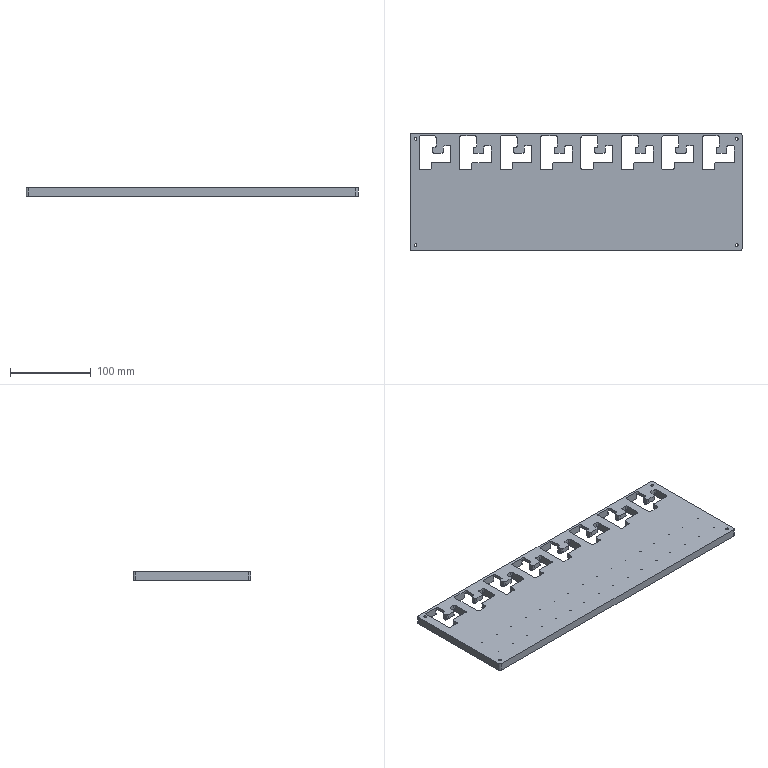NC program | NX | posted with a generic post | part box 410 x 145 x 10 mm
Lines 1 to 26 of 104733:
N10 G17 G21 G94 G90
(FLOOR_WALL , TOOL : D63)
N12 T01 M6
N14 G54
N16 G17 G0 G90 X241.5 Y-72.497 S6500 M3
N18 G43 Z30. H1
N20 Z3.
N22 G94 G1 Z0. F1250.
N24 X238.5
N26 X-238.5
N28 Y-42.548
N30 X238.5
N32 Y-12.599
N34 X-238.5
N36 Y17.351
N38 X238.5
N40 Y47.3
N42 X-238.5
N44 X-241.5
N46 Z3.
N48 G0 Z30.
N50 M5